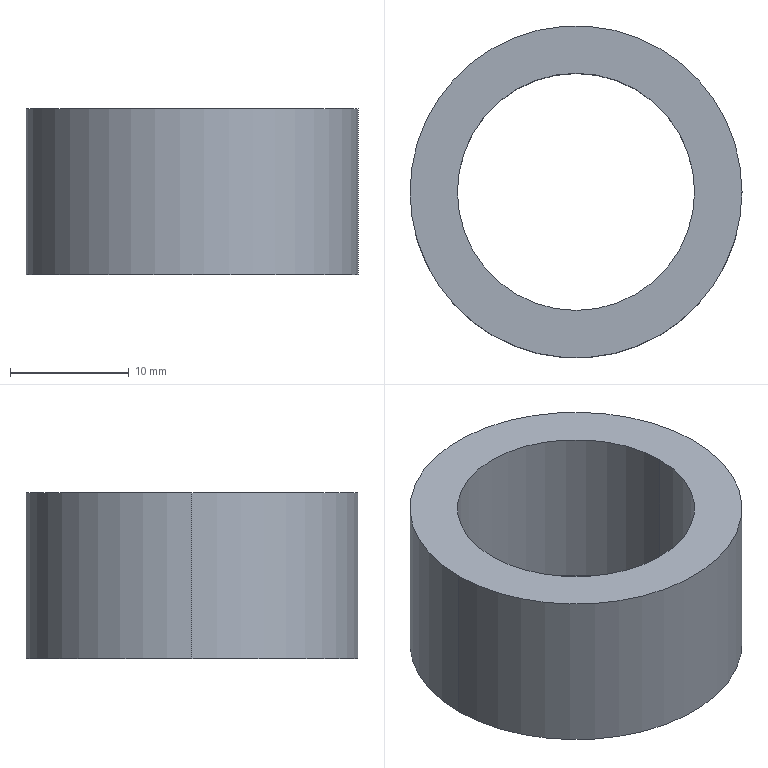Part | STEP file | Pulley end bushing | 1 solid | 6 faces | box 28 x 28 x 14 mm | volume 4222 mm3 | cylinder 4 | plane 2 | commonest cylinder face diameters 20 x2 28 x2
STEP:
#1=CARTESIAN_POINT('',(-10.,0.,14.));
#2=VERTEX_POINT('',#1);
#3=CARTESIAN_POINT('',(10.,0.,14.));
#4=VERTEX_POINT('',#3);
#5=CARTESIAN_POINT('',(0.,0.,14.));
#6=DIRECTION('',(0.,0.,1.));
#7=DIRECTION('',(1.,0.,0.));
#8=AXIS2_PLACEMENT_3D('',#5,#6,#7);
#9=CIRCLE('',#8,10.);
#10=EDGE_CURVE('',#2,#4,#9,.T.);
#11=ORIENTED_EDGE('',*,*,#10,.T.);
#12=CARTESIAN_POINT('',(10.,0.,0.));
#13=VERTEX_POINT('',#12);
#14=CARTESIAN_POINT('',(10.,0.,14.));
#15=DIRECTION('',(0.,0.,-1.));
#16=VECTOR('',#15,1000.);
#17=LINE('',#14,#16);
#18=EDGE_CURVE('',#4,#13,#17,.T.);
#19=ORIENTED_EDGE('',*,*,#18,.T.);
#20=CARTESIAN_POINT('',(-10.,0.,0.));
#21=VERTEX_POINT('',#20);
#22=CARTESIAN_POINT('',(0.,0.,0.));
#23=DIRECTION('',(0.,0.,1.));
#24=DIRECTION('',(1.,0.,0.));
#25=AXIS2_PLACEMENT_3D('',#22,#23,#24);
#26=CIRCLE('',#25,10.);
#27=EDGE_CURVE('',#21,#13,#26,.T.);
#28=ORIENTED_EDGE('',*,*,#27,.F.);
#29=CARTESIAN_POINT('',(-10.,0.,14.));
#30=DIRECTION('',(0.,0.,-1.));
#31=VECTOR('',#30,1000.);
#32=LINE('',#29,#31);
#33=EDGE_CURVE('',#2,#21,#32,.T.);
#34=ORIENTED_EDGE('',*,*,#33,.F.);
#35=EDGE_LOOP('',(#11,#19,#28,#34));
#36=FACE_OUTER_BOUND('',#35,.T.);
#37=CARTESIAN_POINT('',(0.,0.,14.));
#38=DIRECTION('',(0.,0.,-1.));
#39=DIRECTION('',(-1.,0.,0.));
#40=AXIS2_PLACEMENT_3D('',#37,#38,#39);
#41=CYLINDRICAL_SURFACE('',#40,10.);
#42=ADVANCED_FACE('',(#36),#41,.F.);
#43=CARTESIAN_POINT('',(14.,0.,14.));
#44=VERTEX_POINT('',#43);
#45=CARTESIAN_POINT('',(-14.,0.,14.));
#46=VERTEX_POINT('',#45);
#47=CARTESIAN_POINT('',(0.,0.,14.));
#48=DIRECTION('',(0.,0.,1.));
#49=DIRECTION('',(1.,0.,0.));
#50=AXIS2_PLACEMENT_3D('',#47,#48,#49);
#51=CIRCLE('',#50,14.);
#52=EDGE_CURVE('',#44,#46,#51,.T.);
#53=ORIENTED_EDGE('',*,*,#52,.F.);
#54=CARTESIAN_POINT('',(14.,0.,0.));
#55=VERTEX_POINT('',#54);
#56=CARTESIAN_POINT('',(14.,0.,14.));
#57=DIRECTION('',(0.,0.,-1.));
#58=VECTOR('',#57,1000.);
#59=LINE('',#56,#58);
#60=EDGE_CURVE('',#44,#55,#59,.T.);
#61=ORIENTED_EDGE('',*,*,#60,.T.);
#62=CARTESIAN_POINT('',(-14.,0.,0.));
#63=VERTEX_POINT('',#62);
#64=CARTESIAN_POINT('',(0.,0.,0.));
#65=DIRECTION('',(0.,0.,1.));
#66=DIRECTION('',(1.,0.,0.));
#67=AXIS2_PLACEMENT_3D('',#64,#65,#66);
#68=CIRCLE('',#67,14.);
#69=EDGE_CURVE('',#55,#63,#68,.T.);
#70=ORIENTED_EDGE('',*,*,#69,.T.);
#71=CARTESIAN_POINT('',(-14.,0.,14.));
#72=DIRECTION('',(0.,0.,-1.));
#73=VECTOR('',#72,1000.);
#74=LINE('',#71,#73);
#75=EDGE_CURVE('',#46,#63,#74,.T.);
#76=ORIENTED_EDGE('',*,*,#75,.F.);
#77=EDGE_LOOP('',(#53,#61,#70,#76));
#78=FACE_OUTER_BOUND('',#77,.T.);
#79=CARTESIAN_POINT('',(0.,0.,14.));
#80=DIRECTION('',(0.,0.,-1.));
#81=DIRECTION('',(-1.,0.,0.));
#82=AXIS2_PLACEMENT_3D('',#79,#80,#81);
#83=CYLINDRICAL_SURFACE('',#82,14.);
#84=ADVANCED_FACE('',(#78),#83,.T.);
#85=CARTESIAN_POINT('',(0.,0.,14.));
#86=DIRECTION('',(0.,0.,1.));
#87=DIRECTION('',(1.,0.,0.));
#88=AXIS2_PLACEMENT_3D('',#85,#86,#87);
#89=CIRCLE('',#88,14.);
#90=EDGE_CURVE('',#46,#44,#89,.T.);
#91=ORIENTED_EDGE('',*,*,#90,.T.);
#92=ORIENTED_EDGE('',*,*,#52,.T.);
#93=EDGE_LOOP('',(#91,#92));
#94=FACE_OUTER_BOUND('',#93,.T.);
#95=ORIENTED_EDGE('',*,*,#10,.F.);
#96=CARTESIAN_POINT('',(0.,0.,14.));
#97=DIRECTION('',(0.,0.,1.));
#98=DIRECTION('',(1.,0.,0.));
#99=AXIS2_PLACEMENT_3D('',#96,#97,#98);
#100=CIRCLE('',#99,10.);
#101=EDGE_CURVE('',#4,#2,#100,.T.);
#102=ORIENTED_EDGE('',*,*,#101,.F.);
#103=EDGE_LOOP('',(#95,#102));
#104=FACE_BOUND('',#103,.T.);
#105=CARTESIAN_POINT('',(0.,0.,14.));
#106=DIRECTION('',(0.,0.,1.));
#107=DIRECTION('',(1.,0.,0.));
#108=AXIS2_PLACEMENT_3D('',#105,#106,#107);
#109=PLANE('',#108);
#110=ADVANCED_FACE('',(#94,#104),#109,.T.);
#111=CARTESIAN_POINT('',(0.,0.,0.));
#112=DIRECTION('',(0.,0.,1.));
#113=DIRECTION('',(1.,0.,0.));
#114=AXIS2_PLACEMENT_3D('',#111,#112,#113);
#115=CIRCLE('',#114,14.);
#116=EDGE_CURVE('',#63,#55,#115,.T.);
#117=ORIENTED_EDGE('',*,*,#116,.F.);
#118=ORIENTED_EDGE('',*,*,#69,.F.);
#119=EDGE_LOOP('',(#117,#118));
#120=FACE_OUTER_BOUND('',#119,.T.);
#121=ORIENTED_EDGE('',*,*,#27,.T.);
#122=CARTESIAN_POINT('',(0.,0.,0.));
#123=DIRECTION('',(0.,0.,1.));
#124=DIRECTION('',(1.,0.,0.));
#125=AXIS2_PLACEMENT_3D('',#122,#123,#124);
#126=CIRCLE('',#125,10.);
#127=EDGE_CURVE('',#13,#21,#126,.T.);
#128=ORIENTED_EDGE('',*,*,#127,.T.);
#129=EDGE_LOOP('',(#121,#128));
#130=FACE_BOUND('',#129,.T.);
#131=CARTESIAN_POINT('',(0.,0.,0.));
#132=DIRECTION('',(0.,0.,1.));
#133=DIRECTION('',(1.,0.,0.));
#134=AXIS2_PLACEMENT_3D('',#131,#132,#133);
#135=PLANE('',#134);
#136=ADVANCED_FACE('',(#120,#130),#135,.F.);
#137=ORIENTED_EDGE('',*,*,#60,.F.);
#138=ORIENTED_EDGE('',*,*,#90,.F.);
#139=ORIENTED_EDGE('',*,*,#75,.T.);
#140=ORIENTED_EDGE('',*,*,#116,.T.);
#141=EDGE_LOOP('',(#137,#138,#139,#140));
#142=FACE_OUTER_BOUND('',#141,.T.);
#143=CARTESIAN_POINT('',(0.,0.,14.));
#144=DIRECTION('',(0.,0.,-1.));
#145=DIRECTION('',(-1.,0.,0.));
#146=AXIS2_PLACEMENT_3D('',#143,#144,#145);
#147=CYLINDRICAL_SURFACE('',#146,14.);
#148=ADVANCED_FACE('',(#142),#147,.T.);
#149=ORIENTED_EDGE('',*,*,#18,.F.);
#150=ORIENTED_EDGE('',*,*,#101,.T.);
#151=ORIENTED_EDGE('',*,*,#33,.T.);
#152=ORIENTED_EDGE('',*,*,#127,.F.);
#153=EDGE_LOOP('',(#149,#150,#151,#152));
#154=FACE_OUTER_BOUND('',#153,.T.);
#155=CARTESIAN_POINT('',(0.,0.,14.));
#156=DIRECTION('',(0.,0.,-1.));
#157=DIRECTION('',(-1.,0.,0.));
#158=AXIS2_PLACEMENT_3D('',#155,#156,#157);
#159=CYLINDRICAL_SURFACE('',#158,10.);
#160=ADVANCED_FACE('',(#154),#159,.F.);
#161=CLOSED_SHELL('',(#42,#84,#110,#136,#148,#160));
#162=MANIFOLD_SOLID_BREP('',#161);
#163=CARTESIAN_POINT('',(0.,0.,0.));
#164=DIRECTION('',(0.,0.,1.));
#165=DIRECTION('',(1.,0.,0.));
#166=AXIS2_PLACEMENT_3D('',#163,#164,#165);
#167=(LENGTH_UNIT()NAMED_UNIT(*)SI_UNIT(.MILLI.,.METRE.));
#168=UNCERTAINTY_MEASURE_WITH_UNIT(LENGTH_MEASURE(0.00001),#167,'','');
#169=(NAMED_UNIT(*)PLANE_ANGLE_UNIT()SI_UNIT($,.RADIAN.));
#170=(NAMED_UNIT(*)SI_UNIT($,.STERADIAN.)SOLID_ANGLE_UNIT());
#171=(GEOMETRIC_REPRESENTATION_CONTEXT(3)GLOBAL_UNCERTAINTY_ASSIGNED_CONTEXT((#168))GLOBAL_UNIT_ASSIGNED_CONTEXT((#167,#169,#170))REPRESENTATION_CONTEXT('',''));
#172=ADVANCED_BREP_SHAPE_REPRESENTATION('',(#162,#166),#171);